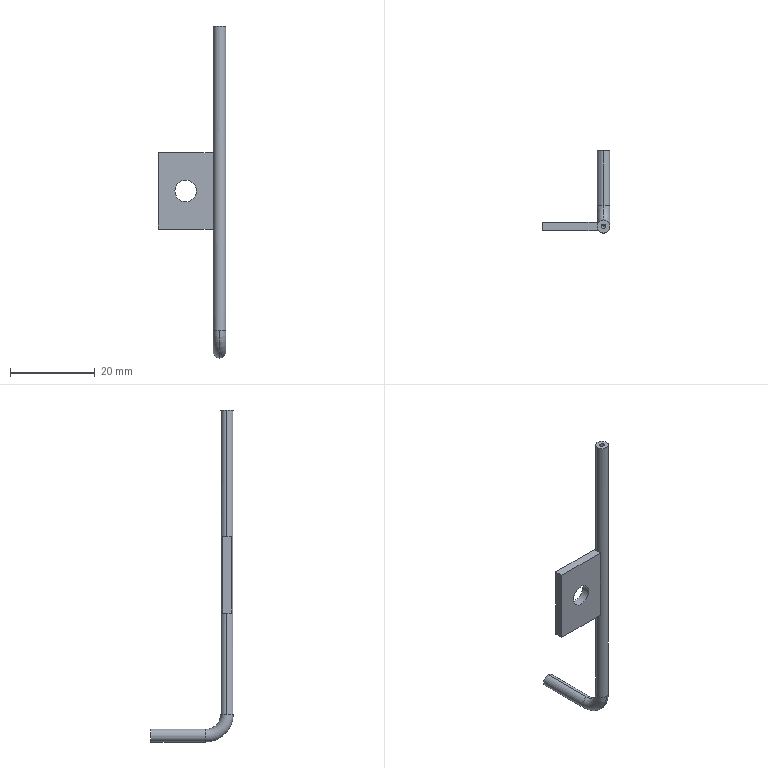Part | NX | features BREP 2 | 2 solids | 22 faces | box 16 x 19.5 x 78.5 mm | volume 1011 mm3 | cylinder 10 | plane 8 | torus 4 | commonest cylinder face diameters 1 x4 3 x4 5.1 x2
STEP:
#1=CARTESIAN_POINT('',(-0.5,0.,-72.));
#2=VERTEX_POINT('',#1);
#3=CARTESIAN_POINT('',(0.,-0.5,-72.));
#4=VERTEX_POINT('',#3);
#5=CARTESIAN_POINT('',(0.,0.,-72.));
#6=DIRECTION('',(0.,0.,1.));
#7=DIRECTION('',(1.,0.,0.));
#8=AXIS2_PLACEMENT_3D('',#5,#6,#7);
#9=CIRCLE('',#8,0.5);
#10=EDGE_CURVE('',#2,#4,#9,.T.);
#11=ORIENTED_EDGE('',*,*,#10,.T.);
#12=CARTESIAN_POINT('',(0.,5.,-77.5));
#13=VERTEX_POINT('',#12);
#14=CARTESIAN_POINT('',(0.,5.,-72.));
#15=DIRECTION('',(1.,0.,0.));
#16=DIRECTION('',(0.,0.,-1.));
#17=AXIS2_PLACEMENT_3D('',#14,#15,#16);
#18=CIRCLE('',#17,5.5);
#19=EDGE_CURVE('',#13,#4,#18,.F.);
#20=ORIENTED_EDGE('',*,*,#19,.F.);
#21=CARTESIAN_POINT('',(0.,5.,-76.5));
#22=VERTEX_POINT('',#21);
#23=CARTESIAN_POINT('',(0.,5.,-77.));
#24=DIRECTION('',(0.,-1.,0.));
#25=DIRECTION('',(1.,0.,0.));
#26=AXIS2_PLACEMENT_3D('',#23,#24,#25);
#27=CIRCLE('',#26,0.5);
#28=EDGE_CURVE('',#22,#13,#27,.T.);
#29=ORIENTED_EDGE('',*,*,#28,.F.);
#30=CARTESIAN_POINT('',(0.,0.5,-72.));
#31=VERTEX_POINT('',#30);
#32=CARTESIAN_POINT('',(0.,5.,-72.));
#33=DIRECTION('',(1.,0.,0.));
#34=DIRECTION('',(0.,0.,-1.));
#35=AXIS2_PLACEMENT_3D('',#32,#33,#34);
#36=CIRCLE('',#35,4.5);
#37=EDGE_CURVE('',#22,#31,#36,.F.);
#38=ORIENTED_EDGE('',*,*,#37,.T.);
#39=CARTESIAN_POINT('',(0.,0.,-72.));
#40=DIRECTION('',(0.,0.,1.));
#41=DIRECTION('',(1.,0.,0.));
#42=AXIS2_PLACEMENT_3D('',#39,#40,#41);
#43=CIRCLE('',#42,0.5);
#44=EDGE_CURVE('',#31,#2,#43,.T.);
#45=ORIENTED_EDGE('',*,*,#44,.T.);
#46=EDGE_LOOP('',(#11,#20,#29,#38,#45));
#47=FACE_BOUND('',#46,.T.);
#48=CARTESIAN_POINT('',(0.,5.,-72.));
#49=DIRECTION('',(1.,0.,0.));
#50=DIRECTION('',(0.,0.,-1.));
#51=AXIS2_PLACEMENT_3D('',#48,#49,#50);
#52=TOROIDAL_SURFACE('',#51,5.,0.5);
#53=ADVANCED_FACE('',(#47),#52,.F.);
#54=CARTESIAN_POINT('',(0.,-1.5,-72.));
#55=VERTEX_POINT('',#54);
#56=CARTESIAN_POINT('',(1.5,0.,-72.));
#57=VERTEX_POINT('',#56);
#58=CARTESIAN_POINT('',(0.,0.,-72.));
#59=DIRECTION('',(0.,0.,1.));
#60=DIRECTION('',(1.,0.,0.));
#61=AXIS2_PLACEMENT_3D('',#58,#59,#60);
#62=CIRCLE('',#61,1.5);
#63=EDGE_CURVE('',#55,#57,#62,.T.);
#64=ORIENTED_EDGE('',*,*,#63,.F.);
#65=CARTESIAN_POINT('',(0.,5.,-78.5));
#66=VERTEX_POINT('',#65);
#67=CARTESIAN_POINT('',(0.,5.,-72.));
#68=DIRECTION('',(1.,0.,0.));
#69=DIRECTION('',(0.,0.,-1.));
#70=AXIS2_PLACEMENT_3D('',#67,#68,#69);
#71=CIRCLE('',#70,6.5);
#72=EDGE_CURVE('',#66,#55,#71,.F.);
#73=ORIENTED_EDGE('',*,*,#72,.F.);
#74=CARTESIAN_POINT('',(0.,5.,-75.5));
#75=VERTEX_POINT('',#74);
#76=CARTESIAN_POINT('',(0.,5.,-77.));
#77=DIRECTION('',(0.,-1.,0.));
#78=DIRECTION('',(1.,0.,0.));
#79=AXIS2_PLACEMENT_3D('',#76,#77,#78);
#80=CIRCLE('',#79,1.5);
#81=EDGE_CURVE('',#66,#75,#80,.T.);
#82=ORIENTED_EDGE('',*,*,#81,.T.);
#83=CARTESIAN_POINT('',(0.,1.5,-72.));
#84=VERTEX_POINT('',#83);
#85=CARTESIAN_POINT('',(0.,5.,-72.));
#86=DIRECTION('',(1.,0.,0.));
#87=DIRECTION('',(0.,0.,-1.));
#88=AXIS2_PLACEMENT_3D('',#85,#86,#87);
#89=CIRCLE('',#88,3.5);
#90=EDGE_CURVE('',#75,#84,#89,.F.);
#91=ORIENTED_EDGE('',*,*,#90,.T.);
#92=CARTESIAN_POINT('',(0.,0.,-72.));
#93=DIRECTION('',(0.,0.,1.));
#94=DIRECTION('',(1.,0.,0.));
#95=AXIS2_PLACEMENT_3D('',#92,#93,#94);
#96=CIRCLE('',#95,1.5);
#97=EDGE_CURVE('',#57,#84,#96,.T.);
#98=ORIENTED_EDGE('',*,*,#97,.F.);
#99=EDGE_LOOP('',(#64,#73,#82,#91,#98));
#100=FACE_BOUND('',#99,.T.);
#101=CARTESIAN_POINT('',(0.,5.,-72.));
#102=DIRECTION('',(1.,0.,0.));
#103=DIRECTION('',(0.,0.,-1.));
#104=AXIS2_PLACEMENT_3D('',#101,#102,#103);
#105=TOROIDAL_SURFACE('',#104,5.,1.5);
#106=ADVANCED_FACE('',(#100),#105,.T.);
#107=ORIENTED_EDGE('',*,*,#97,.T.);
#108=CARTESIAN_POINT('',(-1.5,0.,-72.));
#109=VERTEX_POINT('',#108);
#110=CARTESIAN_POINT('',(0.,0.,-72.));
#111=DIRECTION('',(0.,0.,1.));
#112=DIRECTION('',(1.,0.,0.));
#113=AXIS2_PLACEMENT_3D('',#110,#111,#112);
#114=CIRCLE('',#113,1.5);
#115=EDGE_CURVE('',#84,#109,#114,.T.);
#116=ORIENTED_EDGE('',*,*,#115,.T.);
#117=CARTESIAN_POINT('',(-1.5,0.,0.));
#118=VERTEX_POINT('',#117);
#119=CARTESIAN_POINT('',(-1.5,0.,-72.));
#120=DIRECTION('',(0.,0.,1.));
#121=VECTOR('',#120,1000.);
#122=LINE('',#119,#121);
#123=EDGE_CURVE('',#118,#109,#122,.F.);
#124=ORIENTED_EDGE('',*,*,#123,.F.);
#125=CARTESIAN_POINT('',(1.5,0.,0.));
#126=VERTEX_POINT('',#125);
#127=CARTESIAN_POINT('',(0.,0.,0.));
#128=DIRECTION('',(0.,0.,1.));
#129=DIRECTION('',(1.,0.,0.));
#130=AXIS2_PLACEMENT_3D('',#127,#128,#129);
#131=CIRCLE('',#130,1.5);
#132=EDGE_CURVE('',#126,#118,#131,.T.);
#133=ORIENTED_EDGE('',*,*,#132,.F.);
#134=CARTESIAN_POINT('',(1.5,0.,-72.));
#135=DIRECTION('',(0.,0.,1.));
#136=VECTOR('',#135,1000.);
#137=LINE('',#134,#136);
#138=EDGE_CURVE('',#126,#57,#137,.F.);
#139=ORIENTED_EDGE('',*,*,#138,.T.);
#140=EDGE_LOOP('',(#107,#116,#124,#133,#139));
#141=FACE_BOUND('',#140,.T.);
#142=CARTESIAN_POINT('',(0.,0.,-72.));
#143=DIRECTION('',(0.,0.,1.));
#144=DIRECTION('',(1.,0.,0.));
#145=AXIS2_PLACEMENT_3D('',#142,#143,#144);
#146=CYLINDRICAL_SURFACE('',#145,1.5);
#147=ADVANCED_FACE('',(#141),#146,.T.);
#148=ORIENTED_EDGE('',*,*,#10,.F.);
#149=CARTESIAN_POINT('',(-0.5,0.,0.));
#150=VERTEX_POINT('',#149);
#151=CARTESIAN_POINT('',(-0.5,0.,-72.));
#152=DIRECTION('',(0.,0.,1.));
#153=VECTOR('',#152,1000.);
#154=LINE('',#151,#153);
#155=EDGE_CURVE('',#150,#2,#154,.F.);
#156=ORIENTED_EDGE('',*,*,#155,.F.);
#157=CARTESIAN_POINT('',(0.5,0.,0.));
#158=VERTEX_POINT('',#157);
#159=CARTESIAN_POINT('',(0.,0.,0.));
#160=DIRECTION('',(0.,0.,1.));
#161=DIRECTION('',(1.,0.,0.));
#162=AXIS2_PLACEMENT_3D('',#159,#160,#161);
#163=CIRCLE('',#162,0.5);
#164=EDGE_CURVE('',#150,#158,#163,.T.);
#165=ORIENTED_EDGE('',*,*,#164,.T.);
#166=CARTESIAN_POINT('',(0.5,0.,-72.));
#167=VERTEX_POINT('',#166);
#168=CARTESIAN_POINT('',(0.5,0.,-72.));
#169=DIRECTION('',(0.,0.,1.));
#170=VECTOR('',#169,1000.);
#171=LINE('',#168,#170);
#172=EDGE_CURVE('',#158,#167,#171,.F.);
#173=ORIENTED_EDGE('',*,*,#172,.T.);
#174=CARTESIAN_POINT('',(0.,0.,-72.));
#175=DIRECTION('',(0.,0.,1.));
#176=DIRECTION('',(1.,0.,0.));
#177=AXIS2_PLACEMENT_3D('',#174,#175,#176);
#178=CIRCLE('',#177,0.5);
#179=EDGE_CURVE('',#4,#167,#178,.T.);
#180=ORIENTED_EDGE('',*,*,#179,.F.);
#181=EDGE_LOOP('',(#148,#156,#165,#173,#180));
#182=FACE_BOUND('',#181,.T.);
#183=CARTESIAN_POINT('',(0.,0.,-72.));
#184=DIRECTION('',(0.,0.,1.));
#185=DIRECTION('',(1.,0.,0.));
#186=AXIS2_PLACEMENT_3D('',#183,#184,#185);
#187=CYLINDRICAL_SURFACE('',#186,0.5);
#188=ADVANCED_FACE('',(#182),#187,.F.);
#189=ORIENTED_EDGE('',*,*,#28,.T.);
#190=CARTESIAN_POINT('',(0.,18.,-77.5));
#191=VERTEX_POINT('',#190);
#192=CARTESIAN_POINT('',(0.,5.,-77.5));
#193=DIRECTION('',(0.,1.,0.));
#194=VECTOR('',#193,1000.);
#195=LINE('',#192,#194);
#196=EDGE_CURVE('',#191,#13,#195,.F.);
#197=ORIENTED_EDGE('',*,*,#196,.F.);
#198=CARTESIAN_POINT('',(0.,18.,-76.5));
#199=VERTEX_POINT('',#198);
#200=CARTESIAN_POINT('',(0.,18.,-77.));
#201=DIRECTION('',(0.,-1.,0.));
#202=DIRECTION('',(1.,0.,0.));
#203=AXIS2_PLACEMENT_3D('',#200,#201,#202);
#204=CIRCLE('',#203,0.5);
#205=EDGE_CURVE('',#199,#191,#204,.T.);
#206=ORIENTED_EDGE('',*,*,#205,.F.);
#207=CARTESIAN_POINT('',(0.,5.,-76.5));
#208=DIRECTION('',(0.,1.,0.));
#209=VECTOR('',#208,1000.);
#210=LINE('',#207,#209);
#211=EDGE_CURVE('',#199,#22,#210,.F.);
#212=ORIENTED_EDGE('',*,*,#211,.T.);
#213=EDGE_LOOP('',(#189,#197,#206,#212));
#214=FACE_BOUND('',#213,.T.);
#215=CARTESIAN_POINT('',(0.,5.,-77.));
#216=DIRECTION('',(0.,1.,0.));
#217=DIRECTION('',(0.,0.,1.));
#218=AXIS2_PLACEMENT_3D('',#215,#216,#217);
#219=CYLINDRICAL_SURFACE('',#218,0.5);
#220=ADVANCED_FACE('',(#214),#219,.F.);
#221=ORIENTED_EDGE('',*,*,#81,.F.);
#222=CARTESIAN_POINT('',(0.,18.,-78.5));
#223=VERTEX_POINT('',#222);
#224=CARTESIAN_POINT('',(0.,5.,-78.5));
#225=DIRECTION('',(0.,1.,0.));
#226=VECTOR('',#225,1000.);
#227=LINE('',#224,#226);
#228=EDGE_CURVE('',#223,#66,#227,.F.);
#229=ORIENTED_EDGE('',*,*,#228,.F.);
#230=CARTESIAN_POINT('',(0.,18.,-75.5));
#231=VERTEX_POINT('',#230);
#232=CARTESIAN_POINT('',(0.,18.,-77.));
#233=DIRECTION('',(0.,-1.,0.));
#234=DIRECTION('',(1.,0.,0.));
#235=AXIS2_PLACEMENT_3D('',#232,#233,#234);
#236=CIRCLE('',#235,1.5);
#237=EDGE_CURVE('',#223,#231,#236,.T.);
#238=ORIENTED_EDGE('',*,*,#237,.T.);
#239=CARTESIAN_POINT('',(0.,5.,-75.5));
#240=DIRECTION('',(0.,1.,0.));
#241=VECTOR('',#240,1000.);
#242=LINE('',#239,#241);
#243=EDGE_CURVE('',#231,#75,#242,.F.);
#244=ORIENTED_EDGE('',*,*,#243,.T.);
#245=EDGE_LOOP('',(#221,#229,#238,#244));
#246=FACE_BOUND('',#245,.T.);
#247=CARTESIAN_POINT('',(0.,5.,-77.));
#248=DIRECTION('',(0.,1.,0.));
#249=DIRECTION('',(0.,0.,1.));
#250=AXIS2_PLACEMENT_3D('',#247,#248,#249);
#251=CYLINDRICAL_SURFACE('',#250,1.5);
#252=ADVANCED_FACE('',(#246),#251,.T.);
#253=ORIENTED_EDGE('',*,*,#228,.T.);
#254=CARTESIAN_POINT('',(0.,5.,-77.));
#255=DIRECTION('',(0.,-1.,0.));
#256=DIRECTION('',(1.,0.,0.));
#257=AXIS2_PLACEMENT_3D('',#254,#255,#256);
#258=CIRCLE('',#257,1.5);
#259=EDGE_CURVE('',#75,#66,#258,.T.);
#260=ORIENTED_EDGE('',*,*,#259,.F.);
#261=ORIENTED_EDGE('',*,*,#243,.F.);
#262=CARTESIAN_POINT('',(0.,18.,-77.));
#263=DIRECTION('',(0.,-1.,0.));
#264=DIRECTION('',(1.,0.,0.));
#265=AXIS2_PLACEMENT_3D('',#262,#263,#264);
#266=CIRCLE('',#265,1.5);
#267=EDGE_CURVE('',#231,#223,#266,.T.);
#268=ORIENTED_EDGE('',*,*,#267,.T.);
#269=EDGE_LOOP('',(#253,#260,#261,#268));
#270=FACE_BOUND('',#269,.T.);
#271=CARTESIAN_POINT('',(0.,5.,-77.));
#272=DIRECTION('',(0.,1.,0.));
#273=DIRECTION('',(0.,0.,1.));
#274=AXIS2_PLACEMENT_3D('',#271,#272,#273);
#275=CYLINDRICAL_SURFACE('',#274,1.5);
#276=ADVANCED_FACE('',(#270),#275,.T.);
#277=ORIENTED_EDGE('',*,*,#196,.T.);
#278=CARTESIAN_POINT('',(0.,5.,-77.));
#279=DIRECTION('',(0.,-1.,0.));
#280=DIRECTION('',(1.,0.,0.));
#281=AXIS2_PLACEMENT_3D('',#278,#279,#280);
#282=CIRCLE('',#281,0.5);
#283=EDGE_CURVE('',#13,#22,#282,.T.);
#284=ORIENTED_EDGE('',*,*,#283,.T.);
#285=ORIENTED_EDGE('',*,*,#211,.F.);
#286=CARTESIAN_POINT('',(0.,18.,-77.));
#287=DIRECTION('',(0.,-1.,0.));
#288=DIRECTION('',(1.,0.,0.));
#289=AXIS2_PLACEMENT_3D('',#286,#287,#288);
#290=CIRCLE('',#289,0.5);
#291=EDGE_CURVE('',#191,#199,#290,.T.);
#292=ORIENTED_EDGE('',*,*,#291,.F.);
#293=EDGE_LOOP('',(#277,#284,#285,#292));
#294=FACE_BOUND('',#293,.T.);
#295=CARTESIAN_POINT('',(0.,5.,-77.));
#296=DIRECTION('',(0.,1.,0.));
#297=DIRECTION('',(0.,0.,1.));
#298=AXIS2_PLACEMENT_3D('',#295,#296,#297);
#299=CYLINDRICAL_SURFACE('',#298,0.5);
#300=ADVANCED_FACE('',(#294),#299,.F.);
#301=ORIENTED_EDGE('',*,*,#72,.T.);
#302=CARTESIAN_POINT('',(0.,0.,-72.));
#303=DIRECTION('',(0.,0.,1.));
#304=DIRECTION('',(1.,0.,0.));
#305=AXIS2_PLACEMENT_3D('',#302,#303,#304);
#306=CIRCLE('',#305,1.5);
#307=EDGE_CURVE('',#109,#55,#306,.T.);
#308=ORIENTED_EDGE('',*,*,#307,.F.);
#309=ORIENTED_EDGE('',*,*,#115,.F.);
#310=ORIENTED_EDGE('',*,*,#90,.F.);
#311=ORIENTED_EDGE('',*,*,#259,.T.);
#312=EDGE_LOOP('',(#301,#308,#309,#310,#311));
#313=FACE_BOUND('',#312,.T.);
#314=CARTESIAN_POINT('',(0.,5.,-72.));
#315=DIRECTION('',(1.,0.,0.));
#316=DIRECTION('',(0.,0.,-1.));
#317=AXIS2_PLACEMENT_3D('',#314,#315,#316);
#318=TOROIDAL_SURFACE('',#317,5.,1.5);
#319=ADVANCED_FACE('',(#313),#318,.T.);
#320=ORIENTED_EDGE('',*,*,#19,.T.);
#321=ORIENTED_EDGE('',*,*,#179,.T.);
#322=CARTESIAN_POINT('',(0.,0.,-72.));
#323=DIRECTION('',(0.,0.,1.));
#324=DIRECTION('',(1.,0.,0.));
#325=AXIS2_PLACEMENT_3D('',#322,#323,#324);
#326=CIRCLE('',#325,0.5);
#327=EDGE_CURVE('',#167,#31,#326,.T.);
#328=ORIENTED_EDGE('',*,*,#327,.T.);
#329=ORIENTED_EDGE('',*,*,#37,.F.);
#330=ORIENTED_EDGE('',*,*,#283,.F.);
#331=EDGE_LOOP('',(#320,#321,#328,#329,#330));
#332=FACE_BOUND('',#331,.T.);
#333=CARTESIAN_POINT('',(0.,5.,-72.));
#334=DIRECTION('',(1.,0.,0.));
#335=DIRECTION('',(0.,0.,-1.));
#336=AXIS2_PLACEMENT_3D('',#333,#334,#335);
#337=TOROIDAL_SURFACE('',#336,5.,0.5);
#338=ADVANCED_FACE('',(#332),#337,.F.);
#339=ORIENTED_EDGE('',*,*,#155,.T.);
#340=ORIENTED_EDGE('',*,*,#44,.F.);
#341=ORIENTED_EDGE('',*,*,#327,.F.);
#342=ORIENTED_EDGE('',*,*,#172,.F.);
#343=CARTESIAN_POINT('',(0.,0.,0.));
#344=DIRECTION('',(0.,0.,1.));
#345=DIRECTION('',(1.,0.,0.));
#346=AXIS2_PLACEMENT_3D('',#343,#344,#345);
#347=CIRCLE('',#346,0.5);
#348=EDGE_CURVE('',#158,#150,#347,.T.);
#349=ORIENTED_EDGE('',*,*,#348,.T.);
#350=EDGE_LOOP('',(#339,#340,#341,#342,#349));
#351=FACE_BOUND('',#350,.T.);
#352=CARTESIAN_POINT('',(0.,0.,-72.));
#353=DIRECTION('',(0.,0.,1.));
#354=DIRECTION('',(1.,0.,0.));
#355=AXIS2_PLACEMENT_3D('',#352,#353,#354);
#356=CYLINDRICAL_SURFACE('',#355,0.5);
#357=ADVANCED_FACE('',(#351),#356,.F.);
#358=ORIENTED_EDGE('',*,*,#123,.T.);
#359=ORIENTED_EDGE('',*,*,#307,.T.);
#360=ORIENTED_EDGE('',*,*,#63,.T.);
#361=ORIENTED_EDGE('',*,*,#138,.F.);
#362=CARTESIAN_POINT('',(0.,0.,0.));
#363=DIRECTION('',(0.,0.,1.));
#364=DIRECTION('',(1.,0.,0.));
#365=AXIS2_PLACEMENT_3D('',#362,#363,#364);
#366=CIRCLE('',#365,1.5);
#367=EDGE_CURVE('',#118,#126,#366,.T.);
#368=ORIENTED_EDGE('',*,*,#367,.F.);
#369=EDGE_LOOP('',(#358,#359,#360,#361,#368));
#370=FACE_BOUND('',#369,.T.);
#371=CARTESIAN_POINT('',(0.,0.,-72.));
#372=DIRECTION('',(0.,0.,1.));
#373=DIRECTION('',(1.,0.,0.));
#374=AXIS2_PLACEMENT_3D('',#371,#372,#373);
#375=CYLINDRICAL_SURFACE('',#374,1.5);
#376=ADVANCED_FACE('',(#370),#375,.T.);
#377=ORIENTED_EDGE('',*,*,#267,.F.);
#378=ORIENTED_EDGE('',*,*,#237,.F.);
#379=EDGE_LOOP('',(#377,#378));
#380=FACE_BOUND('',#379,.T.);
#381=ORIENTED_EDGE('',*,*,#205,.T.);
#382=ORIENTED_EDGE('',*,*,#291,.T.);
#383=EDGE_LOOP('',(#381,#382));
#384=FACE_BOUND('',#383,.T.);
#385=CARTESIAN_POINT('',(0.,18.,-77.));
#386=DIRECTION('',(0.,-1.,0.));
#387=DIRECTION('',(0.,0.,-1.));
#388=AXIS2_PLACEMENT_3D('',#385,#386,#387);
#389=PLANE('',#388);
#390=ADVANCED_FACE('',(#380,#384),#389,.F.);
#391=ORIENTED_EDGE('',*,*,#132,.T.);
#392=ORIENTED_EDGE('',*,*,#367,.T.);
#393=EDGE_LOOP('',(#391,#392));
#394=FACE_BOUND('',#393,.T.);
#395=ORIENTED_EDGE('',*,*,#348,.F.);
#396=ORIENTED_EDGE('',*,*,#164,.F.);
#397=EDGE_LOOP('',(#395,#396));
#398=FACE_BOUND('',#397,.T.);
#399=CARTESIAN_POINT('',(0.,0.,0.));
#400=DIRECTION('',(0.,0.,1.));
#401=DIRECTION('',(1.,0.,0.));
#402=AXIS2_PLACEMENT_3D('',#399,#400,#401);
#403=PLANE('',#402);
#404=ADVANCED_FACE('',(#394,#398),#403,.T.);
#405=CLOSED_SHELL('',(#53,#106,#147,#188,#220,#252,#276,#300,#319,#338,#357,#376,#390,#404));
#406=MANIFOLD_SOLID_BREP('',#405);
#407=CARTESIAN_POINT('',(-10.55,1.,-39.));
#408=VERTEX_POINT('',#407);
#409=CARTESIAN_POINT('',(-5.45,1.,-39.));
#410=VERTEX_POINT('',#409);
#411=CARTESIAN_POINT('',(-8.,1.,-39.));
#412=DIRECTION('',(0.,-1.,0.));
#413=DIRECTION('',(0.,0.,-1.));
#414=AXIS2_PLACEMENT_3D('',#411,#412,#413);
#415=CIRCLE('',#414,2.55);
#416=EDGE_CURVE('',#408,#410,#415,.T.);
#417=ORIENTED_EDGE('',*,*,#416,.F.);
#418=CARTESIAN_POINT('',(-10.55,-1.,-39.));
#419=VERTEX_POINT('',#418);
#420=CARTESIAN_POINT('',(-10.55,18.,-39.));
#421=DIRECTION('',(0.,-1.,0.));
#422=VECTOR('',#421,1000.);
#423=LINE('',#420,#422);
#424=EDGE_CURVE('',#419,#408,#423,.F.);
#425=ORIENTED_EDGE('',*,*,#424,.F.);
#426=CARTESIAN_POINT('',(-5.45,-1.,-39.));
#427=VERTEX_POINT('',#426);
#428=CARTESIAN_POINT('',(-8.,-1.,-39.));
#429=DIRECTION('',(0.,-1.,0.));
#430=DIRECTION('',(1.,0.,0.));
#431=AXIS2_PLACEMENT_3D('',#428,#429,#430);
#432=CIRCLE('',#431,2.55);
#433=EDGE_CURVE('',#419,#427,#432,.T.);
#434=ORIENTED_EDGE('',*,*,#433,.T.);
#435=CARTESIAN_POINT('',(-5.45,18.,-39.));
#436=DIRECTION('',(0.,-1.,0.));
#437=VECTOR('',#436,1000.);
#438=LINE('',#435,#437);
#439=EDGE_CURVE('',#427,#410,#438,.F.);
#440=ORIENTED_EDGE('',*,*,#439,.T.);
#441=EDGE_LOOP('',(#417,#425,#434,#440));
#442=FACE_BOUND('',#441,.T.);
#443=CARTESIAN_POINT('',(-8.,18.,-39.));
#444=DIRECTION('',(0.,-1.,0.));
#445=DIRECTION('',(1.,0.,0.));
#446=AXIS2_PLACEMENT_3D('',#443,#444,#445);
#447=CYLINDRICAL_SURFACE('',#446,2.55);
#448=ADVANCED_FACE('',(#442),#447,.F.);
#449=CARTESIAN_POINT('',(-1.5,1.,-30.));
#450=VERTEX_POINT('',#449);
#451=CARTESIAN_POINT('',(-14.5,1.,-30.));
#452=VERTEX_POINT('',#451);
#453=CARTESIAN_POINT('',(-1.5,1.,-30.));
#454=DIRECTION('',(-1.,0.,0.));
#455=VECTOR('',#454,1000.);
#456=LINE('',#453,#455);
#457=EDGE_CURVE('',#450,#452,#456,.T.);
#458=ORIENTED_EDGE('',*,*,#457,.T.);
#459=CARTESIAN_POINT('',(-14.5,-1.,-30.));
#460=VERTEX_POINT('',#459);
#461=CARTESIAN_POINT('',(-14.5,-1.,-30.));
#462=DIRECTION('',(0.,1.,0.));
#463=VECTOR('',#462,1000.);
#464=LINE('',#461,#463);
#465=EDGE_CURVE('',#460,#452,#464,.T.);
#466=ORIENTED_EDGE('',*,*,#465,.F.);
#467=CARTESIAN_POINT('',(-1.5,-1.,-30.));
#468=VERTEX_POINT('',#467);
#469=CARTESIAN_POINT('',(-1.5,-1.,-30.));
#470=DIRECTION('',(-1.,0.,0.));
#471=VECTOR('',#470,1000.);
#472=LINE('',#469,#471);
#473=EDGE_CURVE('',#468,#460,#472,.T.);
#474=ORIENTED_EDGE('',*,*,#473,.F.);
#475=CARTESIAN_POINT('',(-1.5,-1.,-30.));
#476=DIRECTION('',(0.,1.,0.));
#477=VECTOR('',#476,1000.);
#478=LINE('',#475,#477);
#479=EDGE_CURVE('',#468,#450,#478,.T.);
#480=ORIENTED_EDGE('',*,*,#479,.T.);
#481=EDGE_LOOP('',(#458,#466,#474,#480));
#482=FACE_BOUND('',#481,.T.);
#483=CARTESIAN_POINT('',(-1.5,-1.,-30.));
#484=DIRECTION('',(0.,0.,-1.));
#485=DIRECTION('',(0.,-1.,0.));
#486=AXIS2_PLACEMENT_3D('',#483,#484,#485);
#487=PLANE('',#486);
#488=ADVANCED_FACE('',(#482),#487,.F.);
#489=CARTESIAN_POINT('',(-14.5,1.,-48.));
#490=VERTEX_POINT('',#489);
#491=CARTESIAN_POINT('',(-14.5,1.,-30.));
#492=DIRECTION('',(0.,0.,-1.));
#493=VECTOR('',#492,1000.);
#494=LINE('',#491,#493);
#495=EDGE_CURVE('',#452,#490,#494,.T.);
#496=ORIENTED_EDGE('',*,*,#495,.T.);
#497=CARTESIAN_POINT('',(-14.5,-1.,-48.));
#498=VERTEX_POINT('',#497);
#499=CARTESIAN_POINT('',(-14.5,-1.,-48.));
#500=DIRECTION('',(0.,1.,0.));
#501=VECTOR('',#500,1000.);
#502=LINE('',#499,#501);
#503=EDGE_CURVE('',#498,#490,#502,.T.);
#504=ORIENTED_EDGE('',*,*,#503,.F.);
#505=CARTESIAN_POINT('',(-14.5,-1.,-30.));
#506=DIRECTION('',(0.,0.,-1.));
#507=VECTOR('',#506,1000.);
#508=LINE('',#505,#507);
#509=EDGE_CURVE('',#460,#498,#508,.T.);
#510=ORIENTED_EDGE('',*,*,#509,.F.);
#511=ORIENTED_EDGE('',*,*,#465,.T.);
#512=EDGE_LOOP('',(#496,#504,#510,#511));
#513=FACE_BOUND('',#512,.T.);
#514=CARTESIAN_POINT('',(-14.5,-1.,-30.));
#515=DIRECTION('',(1.,0.,0.));
#516=DIRECTION('',(0.,1.,0.));
#517=AXIS2_PLACEMENT_3D('',#514,#515,#516);
#518=PLANE('',#517);
#519=ADVANCED_FACE('',(#513),#518,.F.);
#520=CARTESIAN_POINT('',(-1.5,1.,-48.));
#521=VERTEX_POINT('',#520);
#522=CARTESIAN_POINT('',(-1.5,1.,-48.));
#523=DIRECTION('',(1.,0.,0.));
#524=VECTOR('',#523,1000.);
#525=LINE('',#522,#524);
#526=EDGE_CURVE('',#490,#521,#525,.T.);
#527=ORIENTED_EDGE('',*,*,#526,.T.);
#528=CARTESIAN_POINT('',(-1.5,-1.,-48.));
#529=VERTEX_POINT('',#528);
#530=CARTESIAN_POINT('',(-1.5,-1.,-48.));
#531=DIRECTION('',(0.,1.,0.));
#532=VECTOR('',#531,1000.);
#533=LINE('',#530,#532);
#534=EDGE_CURVE('',#529,#521,#533,.T.);
#535=ORIENTED_EDGE('',*,*,#534,.F.);
#536=CARTESIAN_POINT('',(-1.5,-1.,-48.));
#537=DIRECTION('',(1.,0.,0.));
#538=VECTOR('',#537,1000.);
#539=LINE('',#536,#538);
#540=EDGE_CURVE('',#498,#529,#539,.T.);
#541=ORIENTED_EDGE('',*,*,#540,.F.);
#542=ORIENTED_EDGE('',*,*,#503,.T.);
#543=EDGE_LOOP('',(#527,#535,#541,#542));
#544=FACE_BOUND('',#543,.T.);
#545=CARTESIAN_POINT('',(-1.5,-1.,-48.));
#546=DIRECTION('',(0.,0.,1.));
#547=DIRECTION('',(1.,0.,0.));
#548=AXIS2_PLACEMENT_3D('',#545,#546,#547);
#549=PLANE('',#548);
#550=ADVANCED_FACE('',(#544),#549,.F.);
#551=CARTESIAN_POINT('',(-1.5,1.,-30.));
#552=DIRECTION('',(0.,0.,1.));
#553=VECTOR('',#552,1000.);
#554=LINE('',#551,#553);
#555=EDGE_CURVE('',#521,#450,#554,.T.);
#556=ORIENTED_EDGE('',*,*,#555,.T.);
#557=ORIENTED_EDGE('',*,*,#479,.F.);
#558=CARTESIAN_POINT('',(-1.5,-1.,-30.));
#559=DIRECTION('',(0.,0.,1.));
#560=VECTOR('',#559,1000.);
#561=LINE('',#558,#560);
#562=EDGE_CURVE('',#529,#468,#561,.T.);
#563=ORIENTED_EDGE('',*,*,#562,.F.);
#564=ORIENTED_EDGE('',*,*,#534,.T.);
#565=EDGE_LOOP('',(#556,#557,#563,#564));
#566=FACE_BOUND('',#565,.T.);
#567=CARTESIAN_POINT('',(-1.5,-1.,-30.));
#568=DIRECTION('',(-1.,0.,0.));
#569=DIRECTION('',(0.,0.,1.));
#570=AXIS2_PLACEMENT_3D('',#567,#568,#569);
#571=PLANE('',#570);
#572=ADVANCED_FACE('',(#566),#571,.F.);
#573=ORIENTED_EDGE('',*,*,#473,.T.);
#574=ORIENTED_EDGE('',*,*,#509,.T.);
#575=ORIENTED_EDGE('',*,*,#540,.T.);
#576=ORIENTED_EDGE('',*,*,#562,.T.);
#577=EDGE_LOOP('',(#573,#574,#575,#576));
#578=FACE_BOUND('',#577,.T.);
#579=CARTESIAN_POINT('',(-8.,-1.,-39.));
#580=DIRECTION('',(0.,-1.,0.));
#581=DIRECTION('',(1.,0.,0.));
#582=AXIS2_PLACEMENT_3D('',#579,#580,#581);
#583=CIRCLE('',#582,2.55);
#584=EDGE_CURVE('',#427,#419,#583,.T.);
#585=ORIENTED_EDGE('',*,*,#584,.F.);
#586=ORIENTED_EDGE('',*,*,#433,.F.);
#587=EDGE_LOOP('',(#585,#586));
#588=FACE_BOUND('',#587,.T.);
#589=CARTESIAN_POINT('',(0.,-1.,0.));
#590=DIRECTION('',(0.,-1.,0.));
#591=DIRECTION('',(0.,0.,-1.));
#592=AXIS2_PLACEMENT_3D('',#589,#590,#591);
#593=PLANE('',#592);
#594=ADVANCED_FACE('',(#578,#588),#593,.T.);
#595=ORIENTED_EDGE('',*,*,#457,.F.);
#596=ORIENTED_EDGE('',*,*,#555,.F.);
#597=ORIENTED_EDGE('',*,*,#526,.F.);
#598=ORIENTED_EDGE('',*,*,#495,.F.);
#599=EDGE_LOOP('',(#595,#596,#597,#598));
#600=FACE_BOUND('',#599,.T.);
#601=CARTESIAN_POINT('',(-8.,1.,-39.));
#602=DIRECTION('',(0.,-1.,0.));
#603=DIRECTION('',(0.,0.,-1.));
#604=AXIS2_PLACEMENT_3D('',#601,#602,#603);
#605=CIRCLE('',#604,2.55);
#606=EDGE_CURVE('',#410,#408,#605,.T.);
#607=ORIENTED_EDGE('',*,*,#606,.T.);
#608=ORIENTED_EDGE('',*,*,#416,.T.);
#609=EDGE_LOOP('',(#607,#608));
#610=FACE_BOUND('',#609,.T.);
#611=CARTESIAN_POINT('',(0.,1.,0.));
#612=DIRECTION('',(0.,-1.,0.));
#613=DIRECTION('',(0.,0.,-1.));
#614=AXIS2_PLACEMENT_3D('',#611,#612,#613);
#615=PLANE('',#614);
#616=ADVANCED_FACE('',(#600,#610),#615,.F.);
#617=ORIENTED_EDGE('',*,*,#424,.T.);
#618=ORIENTED_EDGE('',*,*,#606,.F.);
#619=ORIENTED_EDGE('',*,*,#439,.F.);
#620=ORIENTED_EDGE('',*,*,#584,.T.);
#621=EDGE_LOOP('',(#617,#618,#619,#620));
#622=FACE_BOUND('',#621,.T.);
#623=CARTESIAN_POINT('',(-8.,18.,-39.));
#624=DIRECTION('',(0.,-1.,0.));
#625=DIRECTION('',(1.,0.,0.));
#626=AXIS2_PLACEMENT_3D('',#623,#624,#625);
#627=CYLINDRICAL_SURFACE('',#626,2.55);
#628=ADVANCED_FACE('',(#622),#627,.F.);
#629=CLOSED_SHELL('',(#448,#488,#519,#550,#572,#594,#616,#628));
#630=MANIFOLD_SOLID_BREP('',#629);
#631=(LENGTH_UNIT()NAMED_UNIT(*)SI_UNIT(.MILLI.,.METRE.));
#632=UNCERTAINTY_MEASURE_WITH_UNIT(LENGTH_MEASURE(0.00001),#631,'','');
#633=(NAMED_UNIT(*)PLANE_ANGLE_UNIT()SI_UNIT($,.RADIAN.));
#634=(NAMED_UNIT(*)SI_UNIT($,.STERADIAN.)SOLID_ANGLE_UNIT());
#635=(GEOMETRIC_REPRESENTATION_CONTEXT(3)GLOBAL_UNCERTAINTY_ASSIGNED_CONTEXT((#632))GLOBAL_UNIT_ASSIGNED_CONTEXT((#631,#633,#634))REPRESENTATION_CONTEXT('',''));
#636=ADVANCED_BREP_SHAPE_REPRESENTATION('',(#406,#630),#635);